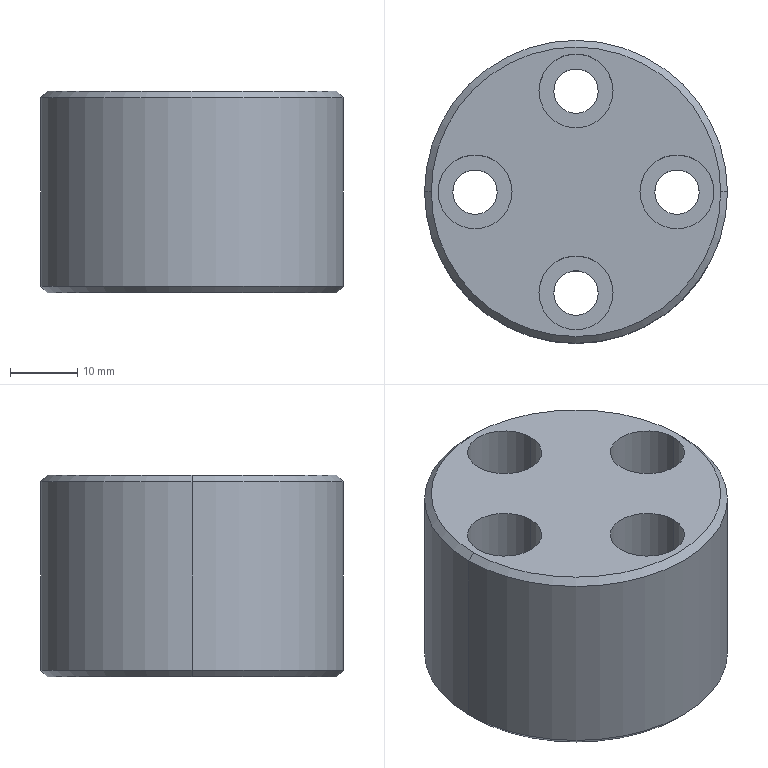Part | STEP file | Locating Pin Seat | 1 solid | 28 faces | box 45 x 45 x 30 mm | volume 38603 mm3 | cylinder 18 | plane 6 | cone 4 | commonest cylinder face diameters 6.6 x8 11 x8 45 x2